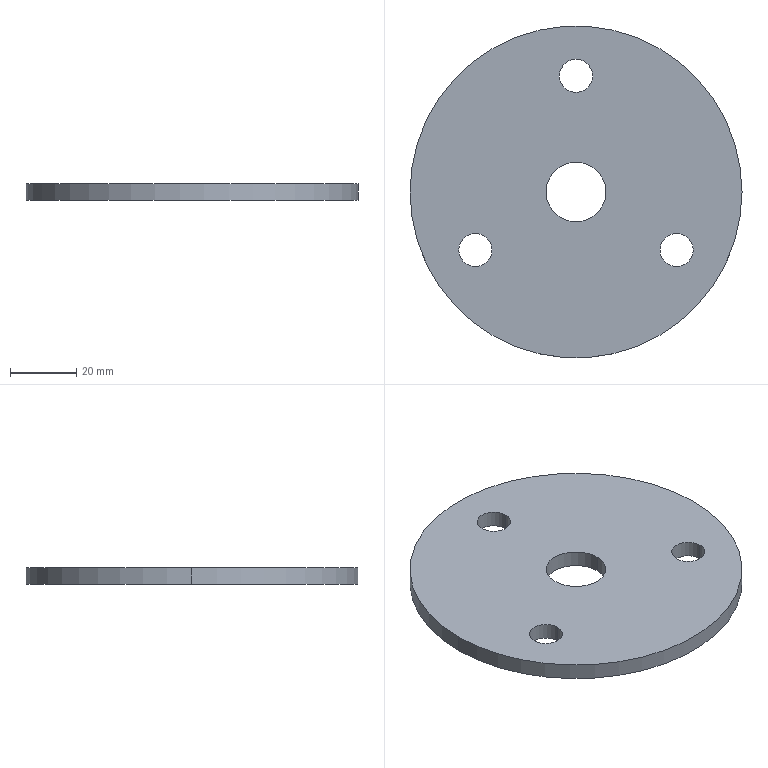Part | SolidWorks | features ICE 2, CirPattern 1, Extrusion 1 | 1 solid | 12 faces | box 100 x 100 x 5 mm | volume 36819 mm3 | cylinder 10 | plane 2 | commonest cylinder face diameters 10 x6 18 x2 100 x2
STEP:
#1=CARTESIAN_POINT('',(-9.,0.,0.));
#2=VERTEX_POINT('',#1);
#3=CARTESIAN_POINT('',(9.,0.,0.));
#4=VERTEX_POINT('',#3);
#5=CARTESIAN_POINT('',(0.,0.,0.));
#6=DIRECTION('',(0.,0.,1.));
#7=DIRECTION('',(1.,0.,0.));
#8=AXIS2_PLACEMENT_3D('',#5,#6,#7);
#9=CIRCLE('',#8,9.);
#10=EDGE_CURVE('',#2,#4,#9,.T.);
#11=ORIENTED_EDGE('',*,*,#10,.F.);
#12=CARTESIAN_POINT('',(-9.,0.,5.));
#13=VERTEX_POINT('',#12);
#14=CARTESIAN_POINT('',(-9.,0.,0.));
#15=DIRECTION('',(0.,0.,1.));
#16=VECTOR('',#15,1000.);
#17=LINE('',#14,#16);
#18=EDGE_CURVE('',#2,#13,#17,.T.);
#19=ORIENTED_EDGE('',*,*,#18,.T.);
#20=CARTESIAN_POINT('',(9.,0.,5.));
#21=VERTEX_POINT('',#20);
#22=CARTESIAN_POINT('',(0.,0.,5.));
#23=DIRECTION('',(0.,0.,1.));
#24=DIRECTION('',(1.,0.,0.));
#25=AXIS2_PLACEMENT_3D('',#22,#23,#24);
#26=CIRCLE('',#25,9.);
#27=EDGE_CURVE('',#13,#21,#26,.T.);
#28=ORIENTED_EDGE('',*,*,#27,.T.);
#29=CARTESIAN_POINT('',(9.,0.,0.));
#30=DIRECTION('',(0.,0.,1.));
#31=VECTOR('',#30,1000.);
#32=LINE('',#29,#31);
#33=EDGE_CURVE('',#4,#21,#32,.T.);
#34=ORIENTED_EDGE('',*,*,#33,.F.);
#35=EDGE_LOOP('',(#11,#19,#28,#34));
#36=FACE_OUTER_BOUND('',#35,.T.);
#37=CARTESIAN_POINT('',(0.,0.,0.));
#38=DIRECTION('',(0.,0.,1.));
#39=DIRECTION('',(1.,0.,0.));
#40=AXIS2_PLACEMENT_3D('',#37,#38,#39);
#41=CYLINDRICAL_SURFACE('',#40,9.);
#42=ADVANCED_FACE('',(#36),#41,.F.);
#43=CARTESIAN_POINT('',(-35.311,-17.5,0.));
#44=VERTEX_POINT('',#43);
#45=CARTESIAN_POINT('',(-25.311,-17.5,0.));
#46=VERTEX_POINT('',#45);
#47=CARTESIAN_POINT('',(-30.311,-17.5,0.));
#48=DIRECTION('',(0.,0.,1.));
#49=DIRECTION('',(-0.5,0.866,0.));
#50=AXIS2_PLACEMENT_3D('',#47,#48,#49);
#51=CIRCLE('',#50,5.);
#52=EDGE_CURVE('',#44,#46,#51,.T.);
#53=ORIENTED_EDGE('',*,*,#52,.F.);
#54=CARTESIAN_POINT('',(-35.311,-17.5,5.));
#55=VERTEX_POINT('',#54);
#56=CARTESIAN_POINT('',(-35.311,-17.5,0.));
#57=DIRECTION('',(0.,0.,1.));
#58=VECTOR('',#57,1000.);
#59=LINE('',#56,#58);
#60=EDGE_CURVE('',#44,#55,#59,.T.);
#61=ORIENTED_EDGE('',*,*,#60,.T.);
#62=CARTESIAN_POINT('',(-25.311,-17.5,5.));
#63=VERTEX_POINT('',#62);
#64=CARTESIAN_POINT('',(-30.311,-17.5,5.));
#65=DIRECTION('',(0.,0.,1.));
#66=DIRECTION('',(-0.5,0.866,0.));
#67=AXIS2_PLACEMENT_3D('',#64,#65,#66);
#68=CIRCLE('',#67,5.);
#69=EDGE_CURVE('',#55,#63,#68,.T.);
#70=ORIENTED_EDGE('',*,*,#69,.T.);
#71=CARTESIAN_POINT('',(-25.311,-17.5,0.));
#72=DIRECTION('',(0.,0.,1.));
#73=VECTOR('',#72,1000.);
#74=LINE('',#71,#73);
#75=EDGE_CURVE('',#46,#63,#74,.T.);
#76=ORIENTED_EDGE('',*,*,#75,.F.);
#77=EDGE_LOOP('',(#53,#61,#70,#76));
#78=FACE_OUTER_BOUND('',#77,.T.);
#79=CARTESIAN_POINT('',(-30.311,-17.5,0.));
#80=DIRECTION('',(0.,0.,1.));
#81=DIRECTION('',(1.,0.,0.));
#82=AXIS2_PLACEMENT_3D('',#79,#80,#81);
#83=CYLINDRICAL_SURFACE('',#82,5.);
#84=ADVANCED_FACE('',(#78),#83,.F.);
#85=CARTESIAN_POINT('',(25.311,-17.5,0.));
#86=VERTEX_POINT('',#85);
#87=CARTESIAN_POINT('',(35.311,-17.5,0.));
#88=VERTEX_POINT('',#87);
#89=CARTESIAN_POINT('',(30.311,-17.5,0.));
#90=DIRECTION('',(0.,0.,1.));
#91=DIRECTION('',(-0.5,-0.866,0.));
#92=AXIS2_PLACEMENT_3D('',#89,#90,#91);
#93=CIRCLE('',#92,5.);
#94=EDGE_CURVE('',#86,#88,#93,.T.);
#95=ORIENTED_EDGE('',*,*,#94,.F.);
#96=CARTESIAN_POINT('',(25.311,-17.5,5.));
#97=VERTEX_POINT('',#96);
#98=CARTESIAN_POINT('',(25.311,-17.5,0.));
#99=DIRECTION('',(0.,0.,1.));
#100=VECTOR('',#99,1000.);
#101=LINE('',#98,#100);
#102=EDGE_CURVE('',#86,#97,#101,.T.);
#103=ORIENTED_EDGE('',*,*,#102,.T.);
#104=CARTESIAN_POINT('',(35.311,-17.5,5.));
#105=VERTEX_POINT('',#104);
#106=CARTESIAN_POINT('',(30.311,-17.5,5.));
#107=DIRECTION('',(0.,0.,1.));
#108=DIRECTION('',(-0.5,-0.866,0.));
#109=AXIS2_PLACEMENT_3D('',#106,#107,#108);
#110=CIRCLE('',#109,5.);
#111=EDGE_CURVE('',#97,#105,#110,.T.);
#112=ORIENTED_EDGE('',*,*,#111,.T.);
#113=CARTESIAN_POINT('',(35.311,-17.5,0.));
#114=DIRECTION('',(0.,0.,1.));
#115=VECTOR('',#114,1000.);
#116=LINE('',#113,#115);
#117=EDGE_CURVE('',#88,#105,#116,.T.);
#118=ORIENTED_EDGE('',*,*,#117,.F.);
#119=EDGE_LOOP('',(#95,#103,#112,#118));
#120=FACE_OUTER_BOUND('',#119,.T.);
#121=CARTESIAN_POINT('',(30.311,-17.5,0.));
#122=DIRECTION('',(0.,0.,1.));
#123=DIRECTION('',(1.,0.,0.));
#124=AXIS2_PLACEMENT_3D('',#121,#122,#123);
#125=CYLINDRICAL_SURFACE('',#124,5.);
#126=ADVANCED_FACE('',(#120),#125,.F.);
#127=CARTESIAN_POINT('',(-5.,35.,0.));
#128=VERTEX_POINT('',#127);
#129=CARTESIAN_POINT('',(5.,35.,0.));
#130=VERTEX_POINT('',#129);
#131=CARTESIAN_POINT('',(0.,35.,0.));
#132=DIRECTION('',(0.,0.,1.));
#133=DIRECTION('',(1.,0.,0.));
#134=AXIS2_PLACEMENT_3D('',#131,#132,#133);
#135=CIRCLE('',#134,5.);
#136=EDGE_CURVE('',#128,#130,#135,.T.);
#137=ORIENTED_EDGE('',*,*,#136,.F.);
#138=CARTESIAN_POINT('',(-5.,35.,5.));
#139=VERTEX_POINT('',#138);
#140=CARTESIAN_POINT('',(-5.,35.,0.));
#141=DIRECTION('',(0.,0.,1.));
#142=VECTOR('',#141,1000.);
#143=LINE('',#140,#142);
#144=EDGE_CURVE('',#128,#139,#143,.T.);
#145=ORIENTED_EDGE('',*,*,#144,.T.);
#146=CARTESIAN_POINT('',(5.,35.,5.));
#147=VERTEX_POINT('',#146);
#148=CARTESIAN_POINT('',(0.,35.,5.));
#149=DIRECTION('',(0.,0.,1.));
#150=DIRECTION('',(1.,0.,0.));
#151=AXIS2_PLACEMENT_3D('',#148,#149,#150);
#152=CIRCLE('',#151,5.);
#153=EDGE_CURVE('',#139,#147,#152,.T.);
#154=ORIENTED_EDGE('',*,*,#153,.T.);
#155=CARTESIAN_POINT('',(5.,35.,0.));
#156=DIRECTION('',(0.,0.,1.));
#157=VECTOR('',#156,1000.);
#158=LINE('',#155,#157);
#159=EDGE_CURVE('',#130,#147,#158,.T.);
#160=ORIENTED_EDGE('',*,*,#159,.F.);
#161=EDGE_LOOP('',(#137,#145,#154,#160));
#162=FACE_OUTER_BOUND('',#161,.T.);
#163=CARTESIAN_POINT('',(0.,35.,0.));
#164=DIRECTION('',(0.,0.,1.));
#165=DIRECTION('',(1.,0.,0.));
#166=AXIS2_PLACEMENT_3D('',#163,#164,#165);
#167=CYLINDRICAL_SURFACE('',#166,5.);
#168=ADVANCED_FACE('',(#162),#167,.F.);
#169=CARTESIAN_POINT('',(50.,0.,5.));
#170=VERTEX_POINT('',#169);
#171=CARTESIAN_POINT('',(-50.,0.,5.));
#172=VERTEX_POINT('',#171);
#173=CARTESIAN_POINT('',(0.,0.,5.));
#174=DIRECTION('',(0.,0.,1.));
#175=DIRECTION('',(1.,0.,0.));
#176=AXIS2_PLACEMENT_3D('',#173,#174,#175);
#177=CIRCLE('',#176,50.);
#178=EDGE_CURVE('',#170,#172,#177,.T.);
#179=ORIENTED_EDGE('',*,*,#178,.F.);
#180=CARTESIAN_POINT('',(50.,0.,0.));
#181=VERTEX_POINT('',#180);
#182=CARTESIAN_POINT('',(50.,0.,5.));
#183=DIRECTION('',(0.,0.,-1.));
#184=VECTOR('',#183,1000.);
#185=LINE('',#182,#184);
#186=EDGE_CURVE('',#170,#181,#185,.T.);
#187=ORIENTED_EDGE('',*,*,#186,.T.);
#188=CARTESIAN_POINT('',(-50.,0.,0.));
#189=VERTEX_POINT('',#188);
#190=CARTESIAN_POINT('',(0.,0.,0.));
#191=DIRECTION('',(0.,0.,1.));
#192=DIRECTION('',(1.,0.,0.));
#193=AXIS2_PLACEMENT_3D('',#190,#191,#192);
#194=CIRCLE('',#193,50.);
#195=EDGE_CURVE('',#181,#189,#194,.T.);
#196=ORIENTED_EDGE('',*,*,#195,.T.);
#197=CARTESIAN_POINT('',(-50.,0.,5.));
#198=DIRECTION('',(0.,0.,-1.));
#199=VECTOR('',#198,1000.);
#200=LINE('',#197,#199);
#201=EDGE_CURVE('',#172,#189,#200,.T.);
#202=ORIENTED_EDGE('',*,*,#201,.F.);
#203=EDGE_LOOP('',(#179,#187,#196,#202));
#204=FACE_OUTER_BOUND('',#203,.T.);
#205=CARTESIAN_POINT('',(0.,0.,5.));
#206=DIRECTION('',(0.,0.,-1.));
#207=DIRECTION('',(-1.,0.,0.));
#208=AXIS2_PLACEMENT_3D('',#205,#206,#207);
#209=CYLINDRICAL_SURFACE('',#208,50.);
#210=ADVANCED_FACE('',(#204),#209,.T.);
#211=ORIENTED_EDGE('',*,*,#186,.F.);
#212=CARTESIAN_POINT('',(0.,0.,5.));
#213=DIRECTION('',(0.,0.,1.));
#214=DIRECTION('',(1.,0.,0.));
#215=AXIS2_PLACEMENT_3D('',#212,#213,#214);
#216=CIRCLE('',#215,50.);
#217=EDGE_CURVE('',#172,#170,#216,.T.);
#218=ORIENTED_EDGE('',*,*,#217,.F.);
#219=ORIENTED_EDGE('',*,*,#201,.T.);
#220=CARTESIAN_POINT('',(0.,0.,0.));
#221=DIRECTION('',(0.,0.,1.));
#222=DIRECTION('',(1.,0.,0.));
#223=AXIS2_PLACEMENT_3D('',#220,#221,#222);
#224=CIRCLE('',#223,50.);
#225=EDGE_CURVE('',#189,#181,#224,.T.);
#226=ORIENTED_EDGE('',*,*,#225,.T.);
#227=EDGE_LOOP('',(#211,#218,#219,#226));
#228=FACE_OUTER_BOUND('',#227,.T.);
#229=CARTESIAN_POINT('',(0.,0.,5.));
#230=DIRECTION('',(0.,0.,-1.));
#231=DIRECTION('',(-1.,0.,0.));
#232=AXIS2_PLACEMENT_3D('',#229,#230,#231);
#233=CYLINDRICAL_SURFACE('',#232,50.);
#234=ADVANCED_FACE('',(#228),#233,.T.);
#235=CARTESIAN_POINT('',(0.,0.,5.));
#236=DIRECTION('',(0.,0.,1.));
#237=DIRECTION('',(1.,0.,0.));
#238=AXIS2_PLACEMENT_3D('',#235,#236,#237);
#239=CIRCLE('',#238,9.);
#240=EDGE_CURVE('',#21,#13,#239,.T.);
#241=ORIENTED_EDGE('',*,*,#240,.F.);
#242=ORIENTED_EDGE('',*,*,#27,.F.);
#243=EDGE_LOOP('',(#241,#242));
#244=FACE_BOUND('',#243,.T.);
#245=CARTESIAN_POINT('',(-30.311,-17.5,5.));
#246=DIRECTION('',(0.,0.,1.));
#247=DIRECTION('',(-0.5,0.866,0.));
#248=AXIS2_PLACEMENT_3D('',#245,#246,#247);
#249=CIRCLE('',#248,5.);
#250=EDGE_CURVE('',#63,#55,#249,.T.);
#251=ORIENTED_EDGE('',*,*,#250,.F.);
#252=ORIENTED_EDGE('',*,*,#69,.F.);
#253=EDGE_LOOP('',(#251,#252));
#254=FACE_BOUND('',#253,.T.);
#255=CARTESIAN_POINT('',(30.311,-17.5,5.));
#256=DIRECTION('',(0.,0.,1.));
#257=DIRECTION('',(-0.5,-0.866,0.));
#258=AXIS2_PLACEMENT_3D('',#255,#256,#257);
#259=CIRCLE('',#258,5.);
#260=EDGE_CURVE('',#105,#97,#259,.T.);
#261=ORIENTED_EDGE('',*,*,#260,.F.);
#262=ORIENTED_EDGE('',*,*,#111,.F.);
#263=EDGE_LOOP('',(#261,#262));
#264=FACE_BOUND('',#263,.T.);
#265=CARTESIAN_POINT('',(0.,35.,5.));
#266=DIRECTION('',(0.,0.,1.));
#267=DIRECTION('',(1.,0.,0.));
#268=AXIS2_PLACEMENT_3D('',#265,#266,#267);
#269=CIRCLE('',#268,5.);
#270=EDGE_CURVE('',#147,#139,#269,.T.);
#271=ORIENTED_EDGE('',*,*,#270,.F.);
#272=ORIENTED_EDGE('',*,*,#153,.F.);
#273=EDGE_LOOP('',(#271,#272));
#274=FACE_BOUND('',#273,.T.);
#275=ORIENTED_EDGE('',*,*,#217,.T.);
#276=ORIENTED_EDGE('',*,*,#178,.T.);
#277=EDGE_LOOP('',(#275,#276));
#278=FACE_OUTER_BOUND('',#277,.T.);
#279=CARTESIAN_POINT('',(0.,0.,5.));
#280=DIRECTION('',(0.,0.,1.));
#281=DIRECTION('',(1.,0.,0.));
#282=AXIS2_PLACEMENT_3D('',#279,#280,#281);
#283=PLANE('',#282);
#284=ADVANCED_FACE('',(#244,#254,#264,#274,#278),#283,.T.);
#285=CARTESIAN_POINT('',(0.,0.,0.));
#286=DIRECTION('',(0.,0.,1.));
#287=DIRECTION('',(1.,0.,0.));
#288=AXIS2_PLACEMENT_3D('',#285,#286,#287);
#289=CIRCLE('',#288,9.);
#290=EDGE_CURVE('',#4,#2,#289,.T.);
#291=ORIENTED_EDGE('',*,*,#290,.T.);
#292=ORIENTED_EDGE('',*,*,#10,.T.);
#293=EDGE_LOOP('',(#291,#292));
#294=FACE_BOUND('',#293,.T.);
#295=CARTESIAN_POINT('',(-30.311,-17.5,0.));
#296=DIRECTION('',(0.,0.,1.));
#297=DIRECTION('',(-0.5,0.866,0.));
#298=AXIS2_PLACEMENT_3D('',#295,#296,#297);
#299=CIRCLE('',#298,5.);
#300=EDGE_CURVE('',#46,#44,#299,.T.);
#301=ORIENTED_EDGE('',*,*,#300,.T.);
#302=ORIENTED_EDGE('',*,*,#52,.T.);
#303=EDGE_LOOP('',(#301,#302));
#304=FACE_BOUND('',#303,.T.);
#305=CARTESIAN_POINT('',(30.311,-17.5,0.));
#306=DIRECTION('',(0.,0.,1.));
#307=DIRECTION('',(-0.5,-0.866,0.));
#308=AXIS2_PLACEMENT_3D('',#305,#306,#307);
#309=CIRCLE('',#308,5.);
#310=EDGE_CURVE('',#88,#86,#309,.T.);
#311=ORIENTED_EDGE('',*,*,#310,.T.);
#312=ORIENTED_EDGE('',*,*,#94,.T.);
#313=EDGE_LOOP('',(#311,#312));
#314=FACE_BOUND('',#313,.T.);
#315=CARTESIAN_POINT('',(0.,35.,0.));
#316=DIRECTION('',(0.,0.,1.));
#317=DIRECTION('',(1.,0.,0.));
#318=AXIS2_PLACEMENT_3D('',#315,#316,#317);
#319=CIRCLE('',#318,5.);
#320=EDGE_CURVE('',#130,#128,#319,.T.);
#321=ORIENTED_EDGE('',*,*,#320,.T.);
#322=ORIENTED_EDGE('',*,*,#136,.T.);
#323=EDGE_LOOP('',(#321,#322));
#324=FACE_BOUND('',#323,.T.);
#325=ORIENTED_EDGE('',*,*,#225,.F.);
#326=ORIENTED_EDGE('',*,*,#195,.F.);
#327=EDGE_LOOP('',(#325,#326));
#328=FACE_OUTER_BOUND('',#327,.T.);
#329=CARTESIAN_POINT('',(0.,0.,0.));
#330=DIRECTION('',(0.,0.,1.));
#331=DIRECTION('',(1.,0.,0.));
#332=AXIS2_PLACEMENT_3D('',#329,#330,#331);
#333=PLANE('',#332);
#334=ADVANCED_FACE('',(#294,#304,#314,#324,#328),#333,.F.);
#335=ORIENTED_EDGE('',*,*,#144,.F.);
#336=ORIENTED_EDGE('',*,*,#320,.F.);
#337=ORIENTED_EDGE('',*,*,#159,.T.);
#338=ORIENTED_EDGE('',*,*,#270,.T.);
#339=EDGE_LOOP('',(#335,#336,#337,#338));
#340=FACE_OUTER_BOUND('',#339,.T.);
#341=CARTESIAN_POINT('',(0.,35.,0.));
#342=DIRECTION('',(0.,0.,1.));
#343=DIRECTION('',(1.,0.,0.));
#344=AXIS2_PLACEMENT_3D('',#341,#342,#343);
#345=CYLINDRICAL_SURFACE('',#344,5.);
#346=ADVANCED_FACE('',(#340),#345,.F.);
#347=ORIENTED_EDGE('',*,*,#102,.F.);
#348=ORIENTED_EDGE('',*,*,#310,.F.);
#349=ORIENTED_EDGE('',*,*,#117,.T.);
#350=ORIENTED_EDGE('',*,*,#260,.T.);
#351=EDGE_LOOP('',(#347,#348,#349,#350));
#352=FACE_OUTER_BOUND('',#351,.T.);
#353=CARTESIAN_POINT('',(30.311,-17.5,0.));
#354=DIRECTION('',(0.,0.,1.));
#355=DIRECTION('',(1.,0.,0.));
#356=AXIS2_PLACEMENT_3D('',#353,#354,#355);
#357=CYLINDRICAL_SURFACE('',#356,5.);
#358=ADVANCED_FACE('',(#352),#357,.F.);
#359=ORIENTED_EDGE('',*,*,#60,.F.);
#360=ORIENTED_EDGE('',*,*,#300,.F.);
#361=ORIENTED_EDGE('',*,*,#75,.T.);
#362=ORIENTED_EDGE('',*,*,#250,.T.);
#363=EDGE_LOOP('',(#359,#360,#361,#362));
#364=FACE_OUTER_BOUND('',#363,.T.);
#365=CARTESIAN_POINT('',(-30.311,-17.5,0.));
#366=DIRECTION('',(0.,0.,1.));
#367=DIRECTION('',(1.,0.,0.));
#368=AXIS2_PLACEMENT_3D('',#365,#366,#367);
#369=CYLINDRICAL_SURFACE('',#368,5.);
#370=ADVANCED_FACE('',(#364),#369,.F.);
#371=ORIENTED_EDGE('',*,*,#18,.F.);
#372=ORIENTED_EDGE('',*,*,#290,.F.);
#373=ORIENTED_EDGE('',*,*,#33,.T.);
#374=ORIENTED_EDGE('',*,*,#240,.T.);
#375=EDGE_LOOP('',(#371,#372,#373,#374));
#376=FACE_OUTER_BOUND('',#375,.T.);
#377=CARTESIAN_POINT('',(0.,0.,0.));
#378=DIRECTION('',(0.,0.,1.));
#379=DIRECTION('',(1.,0.,0.));
#380=AXIS2_PLACEMENT_3D('',#377,#378,#379);
#381=CYLINDRICAL_SURFACE('',#380,9.);
#382=ADVANCED_FACE('',(#376),#381,.F.);
#383=CLOSED_SHELL('',(#42,#84,#126,#168,#210,#234,#284,#334,#346,#358,#370,#382));
#384=MANIFOLD_SOLID_BREP('',#383);
#385=CARTESIAN_POINT('',(0.,0.,0.));
#386=DIRECTION('',(0.,0.,1.));
#387=DIRECTION('',(1.,0.,0.));
#388=AXIS2_PLACEMENT_3D('',#385,#386,#387);
#389=(LENGTH_UNIT()NAMED_UNIT(*)SI_UNIT(.MILLI.,.METRE.));
#390=UNCERTAINTY_MEASURE_WITH_UNIT(LENGTH_MEASURE(0.00001),#389,'','');
#391=(NAMED_UNIT(*)PLANE_ANGLE_UNIT()SI_UNIT($,.RADIAN.));
#392=(NAMED_UNIT(*)SI_UNIT($,.STERADIAN.)SOLID_ANGLE_UNIT());
#393=(GEOMETRIC_REPRESENTATION_CONTEXT(3)GLOBAL_UNCERTAINTY_ASSIGNED_CONTEXT((#390))GLOBAL_UNIT_ASSIGNED_CONTEXT((#389,#391,#392))REPRESENTATION_CONTEXT('',''));
#394=ADVANCED_BREP_SHAPE_REPRESENTATION('',(#384,#388),#393);